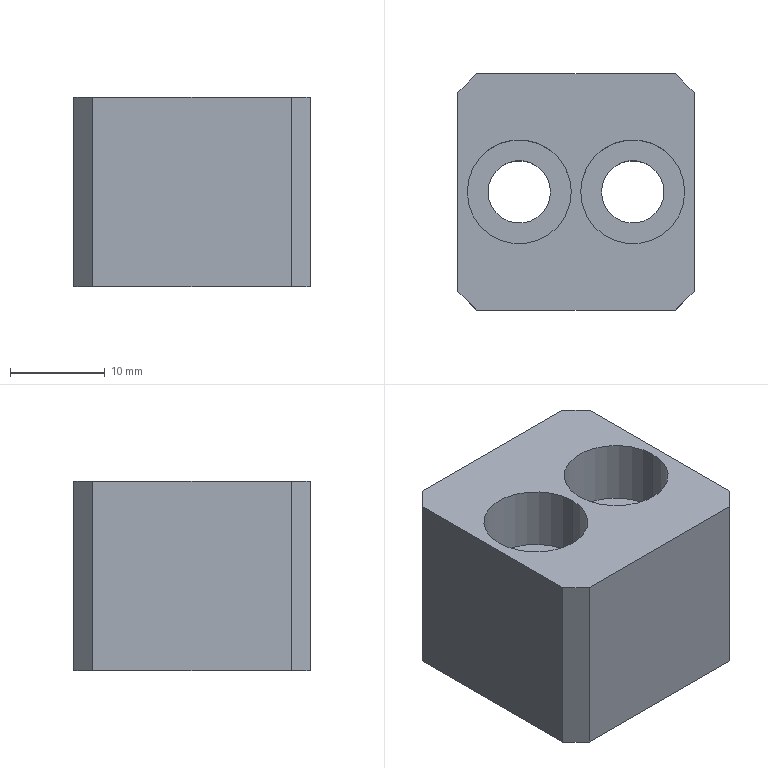Part | STEP file | Magnet block | 1 solid | 20 faces | box 25 x 25 x 20 mm | volume 10144 mm3 | plane 12 | cylinder 8 | commonest cylinder face diameters 6.6 x4 11 x4
STEP:
#1=CARTESIAN_POINT('',(-11.5,0.,13.2));
#2=VERTEX_POINT('',#1);
#3=CARTESIAN_POINT('',(-0.5,0.,13.2));
#4=VERTEX_POINT('',#3);
#5=CARTESIAN_POINT('',(-6.,0.,13.2));
#6=DIRECTION('',(0.,0.,1.));
#7=DIRECTION('',(1.,0.,0.));
#8=AXIS2_PLACEMENT_3D('',#5,#6,#7);
#9=CIRCLE('',#8,5.5);
#10=EDGE_CURVE('',#2,#4,#9,.T.);
#11=ORIENTED_EDGE('',*,*,#10,.F.);
#12=CARTESIAN_POINT('',(-11.5,0.,20.));
#13=VERTEX_POINT('',#12);
#14=CARTESIAN_POINT('',(-11.5,0.,20.));
#15=DIRECTION('',(0.,0.,1.));
#16=VECTOR('',#15,1000.);
#17=LINE('',#14,#16);
#18=EDGE_CURVE('',#2,#13,#17,.T.);
#19=ORIENTED_EDGE('',*,*,#18,.T.);
#20=CARTESIAN_POINT('',(-0.5,0.,20.));
#21=VERTEX_POINT('',#20);
#22=CARTESIAN_POINT('',(-6.,0.,20.));
#23=DIRECTION('',(0.,0.,1.));
#24=DIRECTION('',(1.,0.,0.));
#25=AXIS2_PLACEMENT_3D('',#22,#23,#24);
#26=CIRCLE('',#25,5.5);
#27=EDGE_CURVE('',#13,#21,#26,.T.);
#28=ORIENTED_EDGE('',*,*,#27,.T.);
#29=CARTESIAN_POINT('',(-0.5,0.,20.));
#30=DIRECTION('',(0.,0.,1.));
#31=VECTOR('',#30,1000.);
#32=LINE('',#29,#31);
#33=EDGE_CURVE('',#4,#21,#32,.T.);
#34=ORIENTED_EDGE('',*,*,#33,.F.);
#35=EDGE_LOOP('',(#11,#19,#28,#34));
#36=FACE_OUTER_BOUND('',#35,.T.);
#37=CARTESIAN_POINT('',(-6.,0.,20.));
#38=DIRECTION('',(0.,0.,1.));
#39=DIRECTION('',(1.,0.,0.));
#40=AXIS2_PLACEMENT_3D('',#37,#38,#39);
#41=CYLINDRICAL_SURFACE('',#40,5.5);
#42=ADVANCED_FACE('',(#36),#41,.F.);
#43=CARTESIAN_POINT('',(-9.3,0.,0.));
#44=VERTEX_POINT('',#43);
#45=CARTESIAN_POINT('',(-2.7,0.,0.));
#46=VERTEX_POINT('',#45);
#47=CARTESIAN_POINT('',(-6.,0.,0.));
#48=DIRECTION('',(0.,0.,1.));
#49=DIRECTION('',(1.,0.,0.));
#50=AXIS2_PLACEMENT_3D('',#47,#48,#49);
#51=CIRCLE('',#50,3.3);
#52=EDGE_CURVE('',#44,#46,#51,.T.);
#53=ORIENTED_EDGE('',*,*,#52,.F.);
#54=CARTESIAN_POINT('',(-9.3,0.,13.2));
#55=VERTEX_POINT('',#54);
#56=CARTESIAN_POINT('',(-9.3,0.,20.));
#57=DIRECTION('',(0.,0.,1.));
#58=VECTOR('',#57,1000.);
#59=LINE('',#56,#58);
#60=EDGE_CURVE('',#44,#55,#59,.T.);
#61=ORIENTED_EDGE('',*,*,#60,.T.);
#62=CARTESIAN_POINT('',(-2.7,0.,13.2));
#63=VERTEX_POINT('',#62);
#64=CARTESIAN_POINT('',(-6.,0.,13.2));
#65=DIRECTION('',(0.,0.,1.));
#66=DIRECTION('',(1.,0.,0.));
#67=AXIS2_PLACEMENT_3D('',#64,#65,#66);
#68=CIRCLE('',#67,3.3);
#69=EDGE_CURVE('',#55,#63,#68,.T.);
#70=ORIENTED_EDGE('',*,*,#69,.T.);
#71=CARTESIAN_POINT('',(-2.7,0.,20.));
#72=DIRECTION('',(0.,0.,1.));
#73=VECTOR('',#72,1000.);
#74=LINE('',#71,#73);
#75=EDGE_CURVE('',#46,#63,#74,.T.);
#76=ORIENTED_EDGE('',*,*,#75,.F.);
#77=EDGE_LOOP('',(#53,#61,#70,#76));
#78=FACE_OUTER_BOUND('',#77,.T.);
#79=CARTESIAN_POINT('',(-6.,0.,20.));
#80=DIRECTION('',(0.,0.,1.));
#81=DIRECTION('',(1.,0.,0.));
#82=AXIS2_PLACEMENT_3D('',#79,#80,#81);
#83=CYLINDRICAL_SURFACE('',#82,3.3);
#84=ADVANCED_FACE('',(#78),#83,.F.);
#85=CARTESIAN_POINT('',(0.5,0.,13.2));
#86=VERTEX_POINT('',#85);
#87=CARTESIAN_POINT('',(11.5,0.,13.2));
#88=VERTEX_POINT('',#87);
#89=CARTESIAN_POINT('',(6.,0.,13.2));
#90=DIRECTION('',(0.,0.,1.));
#91=DIRECTION('',(1.,0.,0.));
#92=AXIS2_PLACEMENT_3D('',#89,#90,#91);
#93=CIRCLE('',#92,5.5);
#94=EDGE_CURVE('',#86,#88,#93,.T.);
#95=ORIENTED_EDGE('',*,*,#94,.F.);
#96=CARTESIAN_POINT('',(0.5,0.,20.));
#97=VERTEX_POINT('',#96);
#98=CARTESIAN_POINT('',(0.5,0.,20.));
#99=DIRECTION('',(0.,0.,1.));
#100=VECTOR('',#99,1000.);
#101=LINE('',#98,#100);
#102=EDGE_CURVE('',#86,#97,#101,.T.);
#103=ORIENTED_EDGE('',*,*,#102,.T.);
#104=CARTESIAN_POINT('',(11.5,0.,20.));
#105=VERTEX_POINT('',#104);
#106=CARTESIAN_POINT('',(6.,0.,20.));
#107=DIRECTION('',(0.,0.,1.));
#108=DIRECTION('',(1.,0.,0.));
#109=AXIS2_PLACEMENT_3D('',#106,#107,#108);
#110=CIRCLE('',#109,5.5);
#111=EDGE_CURVE('',#97,#105,#110,.T.);
#112=ORIENTED_EDGE('',*,*,#111,.T.);
#113=CARTESIAN_POINT('',(11.5,0.,20.));
#114=DIRECTION('',(0.,0.,1.));
#115=VECTOR('',#114,1000.);
#116=LINE('',#113,#115);
#117=EDGE_CURVE('',#88,#105,#116,.T.);
#118=ORIENTED_EDGE('',*,*,#117,.F.);
#119=EDGE_LOOP('',(#95,#103,#112,#118));
#120=FACE_OUTER_BOUND('',#119,.T.);
#121=CARTESIAN_POINT('',(6.,0.,20.));
#122=DIRECTION('',(0.,0.,1.));
#123=DIRECTION('',(1.,0.,0.));
#124=AXIS2_PLACEMENT_3D('',#121,#122,#123);
#125=CYLINDRICAL_SURFACE('',#124,5.5);
#126=ADVANCED_FACE('',(#120),#125,.F.);
#127=CARTESIAN_POINT('',(2.7,0.,0.));
#128=VERTEX_POINT('',#127);
#129=CARTESIAN_POINT('',(9.3,0.,0.));
#130=VERTEX_POINT('',#129);
#131=CARTESIAN_POINT('',(6.,0.,0.));
#132=DIRECTION('',(0.,0.,1.));
#133=DIRECTION('',(1.,0.,0.));
#134=AXIS2_PLACEMENT_3D('',#131,#132,#133);
#135=CIRCLE('',#134,3.3);
#136=EDGE_CURVE('',#128,#130,#135,.T.);
#137=ORIENTED_EDGE('',*,*,#136,.F.);
#138=CARTESIAN_POINT('',(2.7,0.,13.2));
#139=VERTEX_POINT('',#138);
#140=CARTESIAN_POINT('',(2.7,0.,20.));
#141=DIRECTION('',(0.,0.,1.));
#142=VECTOR('',#141,1000.);
#143=LINE('',#140,#142);
#144=EDGE_CURVE('',#128,#139,#143,.T.);
#145=ORIENTED_EDGE('',*,*,#144,.T.);
#146=CARTESIAN_POINT('',(9.3,0.,13.2));
#147=VERTEX_POINT('',#146);
#148=CARTESIAN_POINT('',(6.,0.,13.2));
#149=DIRECTION('',(0.,0.,1.));
#150=DIRECTION('',(1.,0.,0.));
#151=AXIS2_PLACEMENT_3D('',#148,#149,#150);
#152=CIRCLE('',#151,3.3);
#153=EDGE_CURVE('',#139,#147,#152,.T.);
#154=ORIENTED_EDGE('',*,*,#153,.T.);
#155=CARTESIAN_POINT('',(9.3,0.,20.));
#156=DIRECTION('',(0.,0.,1.));
#157=VECTOR('',#156,1000.);
#158=LINE('',#155,#157);
#159=EDGE_CURVE('',#130,#147,#158,.T.);
#160=ORIENTED_EDGE('',*,*,#159,.F.);
#161=EDGE_LOOP('',(#137,#145,#154,#160));
#162=FACE_OUTER_BOUND('',#161,.T.);
#163=CARTESIAN_POINT('',(6.,0.,20.));
#164=DIRECTION('',(0.,0.,1.));
#165=DIRECTION('',(1.,0.,0.));
#166=AXIS2_PLACEMENT_3D('',#163,#164,#165);
#167=CYLINDRICAL_SURFACE('',#166,3.3);
#168=ADVANCED_FACE('',(#162),#167,.F.);
#169=CARTESIAN_POINT('',(12.5,-10.5,20.));
#170=VERTEX_POINT('',#169);
#171=CARTESIAN_POINT('',(12.5,10.5,20.));
#172=VERTEX_POINT('',#171);
#173=CARTESIAN_POINT('',(12.5,12.5,20.));
#174=DIRECTION('',(0.,1.,0.));
#175=VECTOR('',#174,1000.);
#176=LINE('',#173,#175);
#177=EDGE_CURVE('',#170,#172,#176,.T.);
#178=ORIENTED_EDGE('',*,*,#177,.F.);
#179=CARTESIAN_POINT('',(12.5,-10.5,0.));
#180=VERTEX_POINT('',#179);
#181=CARTESIAN_POINT('',(12.5,-10.5,20.));
#182=DIRECTION('',(0.,0.,-1.));
#183=VECTOR('',#182,1000.);
#184=LINE('',#181,#183);
#185=EDGE_CURVE('',#170,#180,#184,.T.);
#186=ORIENTED_EDGE('',*,*,#185,.T.);
#187=CARTESIAN_POINT('',(12.5,10.5,0.));
#188=VERTEX_POINT('',#187);
#189=CARTESIAN_POINT('',(12.5,12.5,0.));
#190=DIRECTION('',(0.,1.,0.));
#191=VECTOR('',#190,1000.);
#192=LINE('',#189,#191);
#193=EDGE_CURVE('',#180,#188,#192,.T.);
#194=ORIENTED_EDGE('',*,*,#193,.T.);
#195=CARTESIAN_POINT('',(12.5,10.5,20.));
#196=DIRECTION('',(0.,0.,1.));
#197=VECTOR('',#196,1000.);
#198=LINE('',#195,#197);
#199=EDGE_CURVE('',#188,#172,#198,.T.);
#200=ORIENTED_EDGE('',*,*,#199,.T.);
#201=EDGE_LOOP('',(#178,#186,#194,#200));
#202=FACE_OUTER_BOUND('',#201,.T.);
#203=CARTESIAN_POINT('',(12.5,12.5,20.));
#204=DIRECTION('',(-1.,0.,0.));
#205=DIRECTION('',(0.,0.,1.));
#206=AXIS2_PLACEMENT_3D('',#203,#204,#205);
#207=PLANE('',#206);
#208=ADVANCED_FACE('',(#202),#207,.F.);
#209=CARTESIAN_POINT('',(10.5,12.5,0.));
#210=VERTEX_POINT('',#209);
#211=CARTESIAN_POINT('',(-10.5,12.5,0.));
#212=VERTEX_POINT('',#211);
#213=CARTESIAN_POINT('',(-12.5,12.5,0.));
#214=DIRECTION('',(-1.,0.,0.));
#215=VECTOR('',#214,1000.);
#216=LINE('',#213,#215);
#217=EDGE_CURVE('',#210,#212,#216,.T.);
#218=ORIENTED_EDGE('',*,*,#217,.T.);
#219=CARTESIAN_POINT('',(-10.5,12.5,20.));
#220=VERTEX_POINT('',#219);
#221=CARTESIAN_POINT('',(-10.5,12.5,20.));
#222=DIRECTION('',(0.,0.,1.));
#223=VECTOR('',#222,1000.);
#224=LINE('',#221,#223);
#225=EDGE_CURVE('',#212,#220,#224,.T.);
#226=ORIENTED_EDGE('',*,*,#225,.T.);
#227=CARTESIAN_POINT('',(10.5,12.5,20.));
#228=VERTEX_POINT('',#227);
#229=CARTESIAN_POINT('',(-12.5,12.5,20.));
#230=DIRECTION('',(-1.,0.,0.));
#231=VECTOR('',#230,1000.);
#232=LINE('',#229,#231);
#233=EDGE_CURVE('',#228,#220,#232,.T.);
#234=ORIENTED_EDGE('',*,*,#233,.F.);
#235=CARTESIAN_POINT('',(10.5,12.5,20.));
#236=DIRECTION('',(0.,0.,-1.));
#237=VECTOR('',#236,1000.);
#238=LINE('',#235,#237);
#239=EDGE_CURVE('',#228,#210,#238,.T.);
#240=ORIENTED_EDGE('',*,*,#239,.T.);
#241=EDGE_LOOP('',(#218,#226,#234,#240));
#242=FACE_OUTER_BOUND('',#241,.T.);
#243=CARTESIAN_POINT('',(-12.5,12.5,20.));
#244=DIRECTION('',(0.,-1.,0.));
#245=DIRECTION('',(0.,0.,-1.));
#246=AXIS2_PLACEMENT_3D('',#243,#244,#245);
#247=PLANE('',#246);
#248=ADVANCED_FACE('',(#242),#247,.F.);
#249=CARTESIAN_POINT('',(-12.5,10.5,0.));
#250=VERTEX_POINT('',#249);
#251=CARTESIAN_POINT('',(-12.5,-10.5,0.));
#252=VERTEX_POINT('',#251);
#253=CARTESIAN_POINT('',(-12.5,12.5,0.));
#254=DIRECTION('',(0.,-1.,0.));
#255=VECTOR('',#254,1000.);
#256=LINE('',#253,#255);
#257=EDGE_CURVE('',#250,#252,#256,.T.);
#258=ORIENTED_EDGE('',*,*,#257,.T.);
#259=CARTESIAN_POINT('',(-12.5,-10.5,20.));
#260=VERTEX_POINT('',#259);
#261=CARTESIAN_POINT('',(-12.5,-10.5,20.));
#262=DIRECTION('',(0.,0.,1.));
#263=VECTOR('',#262,1000.);
#264=LINE('',#261,#263);
#265=EDGE_CURVE('',#252,#260,#264,.T.);
#266=ORIENTED_EDGE('',*,*,#265,.T.);
#267=CARTESIAN_POINT('',(-12.5,10.5,20.));
#268=VERTEX_POINT('',#267);
#269=CARTESIAN_POINT('',(-12.5,12.5,20.));
#270=DIRECTION('',(0.,-1.,0.));
#271=VECTOR('',#270,1000.);
#272=LINE('',#269,#271);
#273=EDGE_CURVE('',#268,#260,#272,.T.);
#274=ORIENTED_EDGE('',*,*,#273,.F.);
#275=CARTESIAN_POINT('',(-12.5,10.5,20.));
#276=DIRECTION('',(0.,0.,-1.));
#277=VECTOR('',#276,1000.);
#278=LINE('',#275,#277);
#279=EDGE_CURVE('',#268,#250,#278,.T.);
#280=ORIENTED_EDGE('',*,*,#279,.T.);
#281=EDGE_LOOP('',(#258,#266,#274,#280));
#282=FACE_OUTER_BOUND('',#281,.T.);
#283=CARTESIAN_POINT('',(-12.5,12.5,20.));
#284=DIRECTION('',(1.,0.,0.));
#285=DIRECTION('',(0.,1.,0.));
#286=AXIS2_PLACEMENT_3D('',#283,#284,#285);
#287=PLANE('',#286);
#288=ADVANCED_FACE('',(#282),#287,.F.);
#289=CARTESIAN_POINT('',(-10.5,-12.5,0.));
#290=VERTEX_POINT('',#289);
#291=CARTESIAN_POINT('',(10.5,-12.5,0.));
#292=VERTEX_POINT('',#291);
#293=CARTESIAN_POINT('',(-12.5,-12.5,0.));
#294=DIRECTION('',(1.,0.,0.));
#295=VECTOR('',#294,1000.);
#296=LINE('',#293,#295);
#297=EDGE_CURVE('',#290,#292,#296,.T.);
#298=ORIENTED_EDGE('',*,*,#297,.T.);
#299=CARTESIAN_POINT('',(10.5,-12.5,20.));
#300=VERTEX_POINT('',#299);
#301=CARTESIAN_POINT('',(10.5,-12.5,20.));
#302=DIRECTION('',(0.,0.,1.));
#303=VECTOR('',#302,1000.);
#304=LINE('',#301,#303);
#305=EDGE_CURVE('',#292,#300,#304,.T.);
#306=ORIENTED_EDGE('',*,*,#305,.T.);
#307=CARTESIAN_POINT('',(-10.5,-12.5,20.));
#308=VERTEX_POINT('',#307);
#309=CARTESIAN_POINT('',(-12.5,-12.5,20.));
#310=DIRECTION('',(1.,0.,0.));
#311=VECTOR('',#310,1000.);
#312=LINE('',#309,#311);
#313=EDGE_CURVE('',#308,#300,#312,.T.);
#314=ORIENTED_EDGE('',*,*,#313,.F.);
#315=CARTESIAN_POINT('',(-10.5,-12.5,20.));
#316=DIRECTION('',(0.,0.,-1.));
#317=VECTOR('',#316,1000.);
#318=LINE('',#315,#317);
#319=EDGE_CURVE('',#308,#290,#318,.T.);
#320=ORIENTED_EDGE('',*,*,#319,.T.);
#321=EDGE_LOOP('',(#298,#306,#314,#320));
#322=FACE_OUTER_BOUND('',#321,.T.);
#323=CARTESIAN_POINT('',(-12.5,-12.5,20.));
#324=DIRECTION('',(0.,1.,0.));
#325=DIRECTION('',(0.,0.,1.));
#326=AXIS2_PLACEMENT_3D('',#323,#324,#325);
#327=PLANE('',#326);
#328=ADVANCED_FACE('',(#322),#327,.F.);
#329=CARTESIAN_POINT('',(-6.,0.,20.));
#330=DIRECTION('',(0.,0.,1.));
#331=DIRECTION('',(1.,0.,0.));
#332=AXIS2_PLACEMENT_3D('',#329,#330,#331);
#333=CIRCLE('',#332,5.5);
#334=EDGE_CURVE('',#21,#13,#333,.T.);
#335=ORIENTED_EDGE('',*,*,#334,.F.);
#336=ORIENTED_EDGE('',*,*,#27,.F.);
#337=EDGE_LOOP('',(#335,#336));
#338=FACE_BOUND('',#337,.T.);
#339=CARTESIAN_POINT('',(6.,0.,20.));
#340=DIRECTION('',(0.,0.,1.));
#341=DIRECTION('',(1.,0.,0.));
#342=AXIS2_PLACEMENT_3D('',#339,#340,#341);
#343=CIRCLE('',#342,5.5);
#344=EDGE_CURVE('',#105,#97,#343,.T.);
#345=ORIENTED_EDGE('',*,*,#344,.F.);
#346=ORIENTED_EDGE('',*,*,#111,.F.);
#347=EDGE_LOOP('',(#345,#346));
#348=FACE_BOUND('',#347,.T.);
#349=ORIENTED_EDGE('',*,*,#313,.T.);
#350=CARTESIAN_POINT('',(11.5,-11.5,20.));
#351=DIRECTION('',(0.7071,0.7071,0.));
#352=VECTOR('',#351,1000.);
#353=LINE('',#350,#352);
#354=EDGE_CURVE('',#300,#170,#353,.T.);
#355=ORIENTED_EDGE('',*,*,#354,.T.);
#356=ORIENTED_EDGE('',*,*,#177,.T.);
#357=CARTESIAN_POINT('',(11.5,11.5,20.));
#358=DIRECTION('',(-0.7071,0.7071,0.));
#359=VECTOR('',#358,1000.);
#360=LINE('',#357,#359);
#361=EDGE_CURVE('',#172,#228,#360,.T.);
#362=ORIENTED_EDGE('',*,*,#361,.T.);
#363=ORIENTED_EDGE('',*,*,#233,.T.);
#364=CARTESIAN_POINT('',(-11.5,11.5,20.));
#365=DIRECTION('',(-0.7071,-0.7071,0.));
#366=VECTOR('',#365,1000.);
#367=LINE('',#364,#366);
#368=EDGE_CURVE('',#220,#268,#367,.T.);
#369=ORIENTED_EDGE('',*,*,#368,.T.);
#370=ORIENTED_EDGE('',*,*,#273,.T.);
#371=CARTESIAN_POINT('',(-11.5,-11.5,20.));
#372=DIRECTION('',(0.7071,-0.7071,0.));
#373=VECTOR('',#372,1000.);
#374=LINE('',#371,#373);
#375=EDGE_CURVE('',#260,#308,#374,.T.);
#376=ORIENTED_EDGE('',*,*,#375,.T.);
#377=EDGE_LOOP('',(#349,#355,#356,#362,#363,#369,#370,#376));
#378=FACE_OUTER_BOUND('',#377,.T.);
#379=CARTESIAN_POINT('',(0.,0.,20.));
#380=DIRECTION('',(0.,0.,1.));
#381=DIRECTION('',(1.,0.,0.));
#382=AXIS2_PLACEMENT_3D('',#379,#380,#381);
#383=PLANE('',#382);
#384=ADVANCED_FACE('',(#338,#348,#378),#383,.T.);
#385=CARTESIAN_POINT('',(-6.,0.,0.));
#386=DIRECTION('',(0.,0.,1.));
#387=DIRECTION('',(1.,0.,0.));
#388=AXIS2_PLACEMENT_3D('',#385,#386,#387);
#389=CIRCLE('',#388,3.3);
#390=EDGE_CURVE('',#46,#44,#389,.T.);
#391=ORIENTED_EDGE('',*,*,#390,.T.);
#392=ORIENTED_EDGE('',*,*,#52,.T.);
#393=EDGE_LOOP('',(#391,#392));
#394=FACE_BOUND('',#393,.T.);
#395=CARTESIAN_POINT('',(6.,0.,0.));
#396=DIRECTION('',(0.,0.,1.));
#397=DIRECTION('',(1.,0.,0.));
#398=AXIS2_PLACEMENT_3D('',#395,#396,#397);
#399=CIRCLE('',#398,3.3);
#400=EDGE_CURVE('',#130,#128,#399,.T.);
#401=ORIENTED_EDGE('',*,*,#400,.T.);
#402=ORIENTED_EDGE('',*,*,#136,.T.);
#403=EDGE_LOOP('',(#401,#402));
#404=FACE_BOUND('',#403,.T.);
#405=ORIENTED_EDGE('',*,*,#193,.F.);
#406=CARTESIAN_POINT('',(12.5,-10.5,0.));
#407=DIRECTION('',(-0.7071,-0.7071,0.));
#408=VECTOR('',#407,1000.);
#409=LINE('',#406,#408);
#410=EDGE_CURVE('',#180,#292,#409,.T.);
#411=ORIENTED_EDGE('',*,*,#410,.T.);
#412=ORIENTED_EDGE('',*,*,#297,.F.);
#413=CARTESIAN_POINT('',(-10.5,-12.5,0.));
#414=DIRECTION('',(-0.7071,0.7071,0.));
#415=VECTOR('',#414,1000.);
#416=LINE('',#413,#415);
#417=EDGE_CURVE('',#290,#252,#416,.T.);
#418=ORIENTED_EDGE('',*,*,#417,.T.);
#419=ORIENTED_EDGE('',*,*,#257,.F.);
#420=CARTESIAN_POINT('',(-12.5,10.5,0.));
#421=DIRECTION('',(0.7071,0.7071,0.));
#422=VECTOR('',#421,1000.);
#423=LINE('',#420,#422);
#424=EDGE_CURVE('',#250,#212,#423,.T.);
#425=ORIENTED_EDGE('',*,*,#424,.T.);
#426=ORIENTED_EDGE('',*,*,#217,.F.);
#427=CARTESIAN_POINT('',(10.5,12.5,0.));
#428=DIRECTION('',(0.7071,-0.7071,0.));
#429=VECTOR('',#428,1000.);
#430=LINE('',#427,#429);
#431=EDGE_CURVE('',#210,#188,#430,.T.);
#432=ORIENTED_EDGE('',*,*,#431,.T.);
#433=EDGE_LOOP('',(#405,#411,#412,#418,#419,#425,#426,#432));
#434=FACE_OUTER_BOUND('',#433,.T.);
#435=CARTESIAN_POINT('',(0.,0.,0.));
#436=DIRECTION('',(0.,0.,1.));
#437=DIRECTION('',(1.,0.,0.));
#438=AXIS2_PLACEMENT_3D('',#435,#436,#437);
#439=PLANE('',#438);
#440=ADVANCED_FACE('',(#394,#404,#434),#439,.F.);
#441=ORIENTED_EDGE('',*,*,#144,.F.);
#442=ORIENTED_EDGE('',*,*,#400,.F.);
#443=ORIENTED_EDGE('',*,*,#159,.T.);
#444=CARTESIAN_POINT('',(6.,0.,13.2));
#445=DIRECTION('',(0.,0.,1.));
#446=DIRECTION('',(1.,0.,0.));
#447=AXIS2_PLACEMENT_3D('',#444,#445,#446);
#448=CIRCLE('',#447,3.3);
#449=EDGE_CURVE('',#147,#139,#448,.T.);
#450=ORIENTED_EDGE('',*,*,#449,.T.);
#451=EDGE_LOOP('',(#441,#442,#443,#450));
#452=FACE_OUTER_BOUND('',#451,.T.);
#453=CARTESIAN_POINT('',(6.,0.,20.));
#454=DIRECTION('',(0.,0.,1.));
#455=DIRECTION('',(1.,0.,0.));
#456=AXIS2_PLACEMENT_3D('',#453,#454,#455);
#457=CYLINDRICAL_SURFACE('',#456,3.3);
#458=ADVANCED_FACE('',(#452),#457,.F.);
#459=ORIENTED_EDGE('',*,*,#449,.F.);
#460=ORIENTED_EDGE('',*,*,#153,.F.);
#461=EDGE_LOOP('',(#459,#460));
#462=FACE_BOUND('',#461,.T.);
#463=CARTESIAN_POINT('',(6.,0.,13.2));
#464=DIRECTION('',(0.,0.,1.));
#465=DIRECTION('',(1.,0.,0.));
#466=AXIS2_PLACEMENT_3D('',#463,#464,#465);
#467=CIRCLE('',#466,5.5);
#468=EDGE_CURVE('',#88,#86,#467,.T.);
#469=ORIENTED_EDGE('',*,*,#468,.T.);
#470=ORIENTED_EDGE('',*,*,#94,.T.);
#471=EDGE_LOOP('',(#469,#470));
#472=FACE_OUTER_BOUND('',#471,.T.);
#473=CARTESIAN_POINT('',(9.3,0.,13.2));
#474=DIRECTION('',(0.,0.,-1.));
#475=DIRECTION('',(-1.,0.,0.));
#476=AXIS2_PLACEMENT_3D('',#473,#474,#475);
#477=PLANE('',#476);
#478=ADVANCED_FACE('',(#462,#472),#477,.F.);
#479=ORIENTED_EDGE('',*,*,#102,.F.);
#480=ORIENTED_EDGE('',*,*,#468,.F.);
#481=ORIENTED_EDGE('',*,*,#117,.T.);
#482=ORIENTED_EDGE('',*,*,#344,.T.);
#483=EDGE_LOOP('',(#479,#480,#481,#482));
#484=FACE_OUTER_BOUND('',#483,.T.);
#485=CARTESIAN_POINT('',(6.,0.,20.));
#486=DIRECTION('',(0.,0.,1.));
#487=DIRECTION('',(1.,0.,0.));
#488=AXIS2_PLACEMENT_3D('',#485,#486,#487);
#489=CYLINDRICAL_SURFACE('',#488,5.5);
#490=ADVANCED_FACE('',(#484),#489,.F.);
#491=ORIENTED_EDGE('',*,*,#60,.F.);
#492=ORIENTED_EDGE('',*,*,#390,.F.);
#493=ORIENTED_EDGE('',*,*,#75,.T.);
#494=CARTESIAN_POINT('',(-6.,0.,13.2));
#495=DIRECTION('',(0.,0.,1.));
#496=DIRECTION('',(1.,0.,0.));
#497=AXIS2_PLACEMENT_3D('',#494,#495,#496);
#498=CIRCLE('',#497,3.3);
#499=EDGE_CURVE('',#63,#55,#498,.T.);
#500=ORIENTED_EDGE('',*,*,#499,.T.);
#501=EDGE_LOOP('',(#491,#492,#493,#500));
#502=FACE_OUTER_BOUND('',#501,.T.);
#503=CARTESIAN_POINT('',(-6.,0.,20.));
#504=DIRECTION('',(0.,0.,1.));
#505=DIRECTION('',(1.,0.,0.));
#506=AXIS2_PLACEMENT_3D('',#503,#504,#505);
#507=CYLINDRICAL_SURFACE('',#506,3.3);
#508=ADVANCED_FACE('',(#502),#507,.F.);
#509=ORIENTED_EDGE('',*,*,#499,.F.);
#510=ORIENTED_EDGE('',*,*,#69,.F.);
#511=EDGE_LOOP('',(#509,#510));
#512=FACE_BOUND('',#511,.T.);
#513=CARTESIAN_POINT('',(-6.,0.,13.2));
#514=DIRECTION('',(0.,0.,1.));
#515=DIRECTION('',(1.,0.,0.));
#516=AXIS2_PLACEMENT_3D('',#513,#514,#515);
#517=CIRCLE('',#516,5.5);
#518=EDGE_CURVE('',#4,#2,#517,.T.);
#519=ORIENTED_EDGE('',*,*,#518,.T.);
#520=ORIENTED_EDGE('',*,*,#10,.T.);
#521=EDGE_LOOP('',(#519,#520));
#522=FACE_OUTER_BOUND('',#521,.T.);
#523=CARTESIAN_POINT('',(-2.7,0.,13.2));
#524=DIRECTION('',(0.,0.,-1.));
#525=DIRECTION('',(-1.,0.,0.));
#526=AXIS2_PLACEMENT_3D('',#523,#524,#525);
#527=PLANE('',#526);
#528=ADVANCED_FACE('',(#512,#522),#527,.F.);
#529=ORIENTED_EDGE('',*,*,#18,.F.);
#530=ORIENTED_EDGE('',*,*,#518,.F.);
#531=ORIENTED_EDGE('',*,*,#33,.T.);
#532=ORIENTED_EDGE('',*,*,#334,.T.);
#533=EDGE_LOOP('',(#529,#530,#531,#532));
#534=FACE_OUTER_BOUND('',#533,.T.);
#535=CARTESIAN_POINT('',(-6.,0.,20.));
#536=DIRECTION('',(0.,0.,1.));
#537=DIRECTION('',(1.,0.,0.));
#538=AXIS2_PLACEMENT_3D('',#535,#536,#537);
#539=CYLINDRICAL_SURFACE('',#538,5.5);
#540=ADVANCED_FACE('',(#534),#539,.F.);
#541=ORIENTED_EDGE('',*,*,#354,.F.);
#542=ORIENTED_EDGE('',*,*,#305,.F.);
#543=ORIENTED_EDGE('',*,*,#410,.F.);
#544=ORIENTED_EDGE('',*,*,#185,.F.);
#545=EDGE_LOOP('',(#541,#542,#543,#544));
#546=FACE_OUTER_BOUND('',#545,.T.);
#547=CARTESIAN_POINT('',(12.5,-10.5,20.));
#548=DIRECTION('',(-0.7071,0.7071,0.));
#549=DIRECTION('',(0.,0.,-1.));
#550=AXIS2_PLACEMENT_3D('',#547,#548,#549);
#551=PLANE('',#550);
#552=ADVANCED_FACE('',(#546),#551,.F.);
#553=ORIENTED_EDGE('',*,*,#375,.F.);
#554=ORIENTED_EDGE('',*,*,#265,.F.);
#555=ORIENTED_EDGE('',*,*,#417,.F.);
#556=ORIENTED_EDGE('',*,*,#319,.F.);
#557=EDGE_LOOP('',(#553,#554,#555,#556));
#558=FACE_OUTER_BOUND('',#557,.T.);
#559=CARTESIAN_POINT('',(-10.5,-12.5,20.));
#560=DIRECTION('',(0.7071,0.7071,0.));
#561=DIRECTION('',(0.,0.,-1.));
#562=AXIS2_PLACEMENT_3D('',#559,#560,#561);
#563=PLANE('',#562);
#564=ADVANCED_FACE('',(#558),#563,.F.);
#565=ORIENTED_EDGE('',*,*,#368,.F.);
#566=ORIENTED_EDGE('',*,*,#225,.F.);
#567=ORIENTED_EDGE('',*,*,#424,.F.);
#568=ORIENTED_EDGE('',*,*,#279,.F.);
#569=EDGE_LOOP('',(#565,#566,#567,#568));
#570=FACE_OUTER_BOUND('',#569,.T.);
#571=CARTESIAN_POINT('',(-12.5,10.5,20.));
#572=DIRECTION('',(0.7071,-0.7071,0.));
#573=DIRECTION('',(0.,0.,-1.));
#574=AXIS2_PLACEMENT_3D('',#571,#572,#573);
#575=PLANE('',#574);
#576=ADVANCED_FACE('',(#570),#575,.F.);
#577=ORIENTED_EDGE('',*,*,#361,.F.);
#578=ORIENTED_EDGE('',*,*,#199,.F.);
#579=ORIENTED_EDGE('',*,*,#431,.F.);
#580=ORIENTED_EDGE('',*,*,#239,.F.);
#581=EDGE_LOOP('',(#577,#578,#579,#580));
#582=FACE_OUTER_BOUND('',#581,.T.);
#583=CARTESIAN_POINT('',(10.5,12.5,20.));
#584=DIRECTION('',(-0.7071,-0.7071,0.));
#585=DIRECTION('',(0.,0.,-1.));
#586=AXIS2_PLACEMENT_3D('',#583,#584,#585);
#587=PLANE('',#586);
#588=ADVANCED_FACE('',(#582),#587,.F.);
#589=CLOSED_SHELL('',(#42,#84,#126,#168,#208,#248,#288,#328,#384,#440,#458,#478,#490,#508,#528,#540,#552,#564,#576,#588));
#590=MANIFOLD_SOLID_BREP('',#589);
#591=CARTESIAN_POINT('',(0.,0.,0.));
#592=DIRECTION('',(0.,0.,1.));
#593=DIRECTION('',(1.,0.,0.));
#594=AXIS2_PLACEMENT_3D('',#591,#592,#593);
#595=(LENGTH_UNIT()NAMED_UNIT(*)SI_UNIT(.MILLI.,.METRE.));
#596=UNCERTAINTY_MEASURE_WITH_UNIT(LENGTH_MEASURE(0.00001),#595,'','');
#597=(NAMED_UNIT(*)PLANE_ANGLE_UNIT()SI_UNIT($,.RADIAN.));
#598=(NAMED_UNIT(*)SI_UNIT($,.STERADIAN.)SOLID_ANGLE_UNIT());
#599=(GEOMETRIC_REPRESENTATION_CONTEXT(3)GLOBAL_UNCERTAINTY_ASSIGNED_CONTEXT((#596))GLOBAL_UNIT_ASSIGNED_CONTEXT((#595,#597,#598))REPRESENTATION_CONTEXT('',''));
#600=ADVANCED_BREP_SHAPE_REPRESENTATION('',(#590,#594),#599);